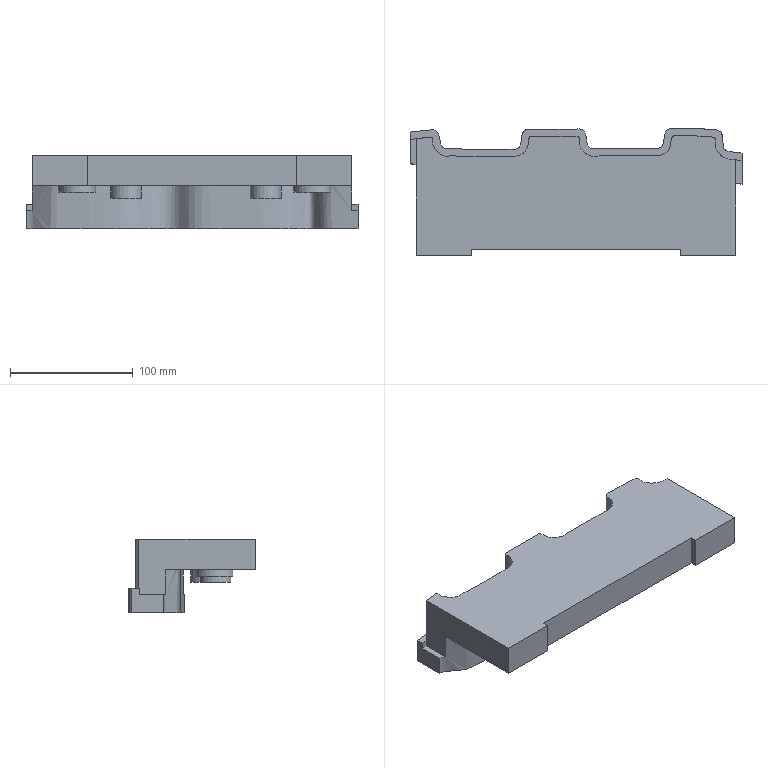Part | NX | features solid 2 | 1 solid | 28 faces | box 270 x 103.259 x 60 mm | volume 729885 mm3 | plane 18 | spline 6 | cylinder 4 | commonest cylinder face diameters 25 x2 30 x2